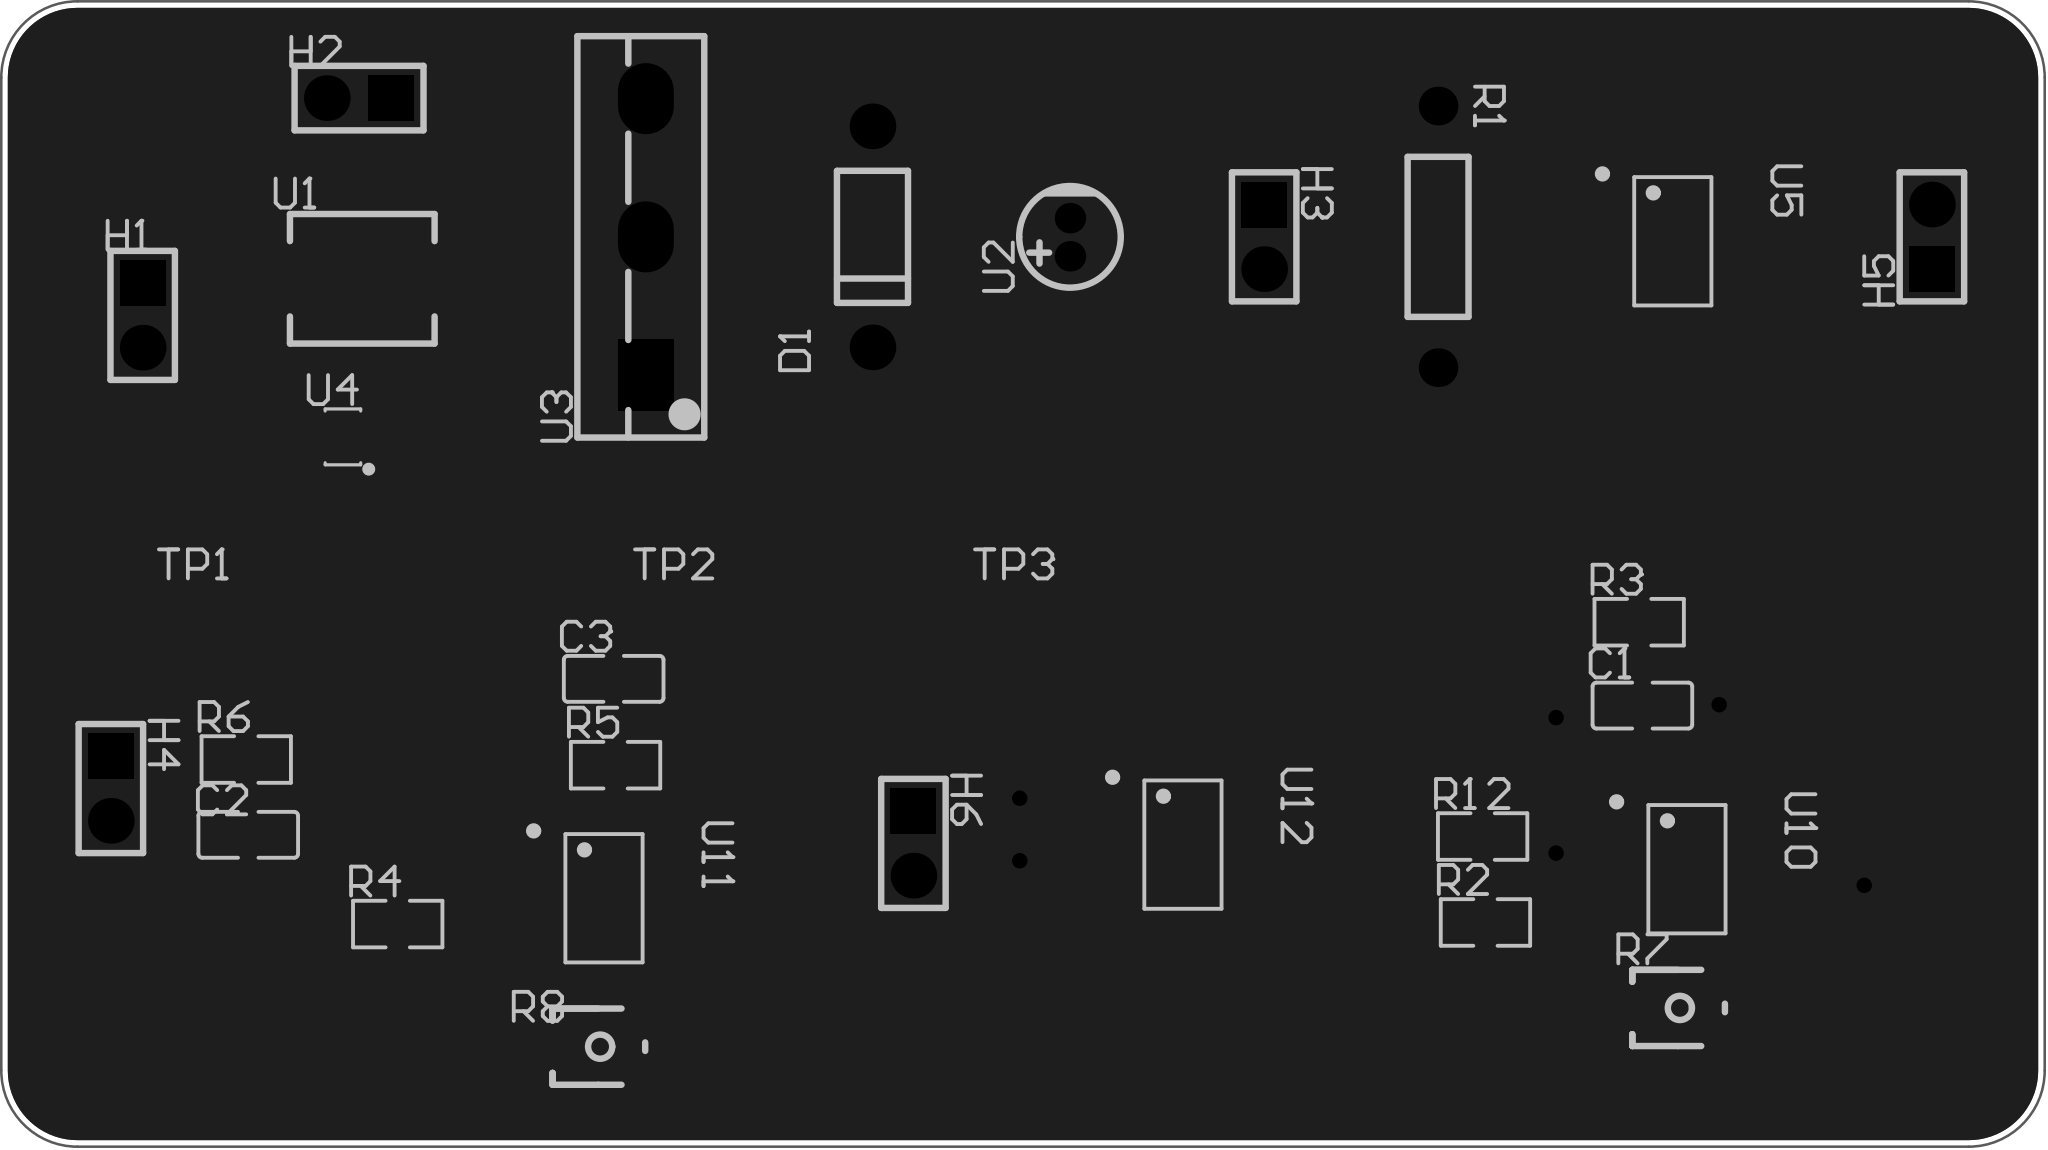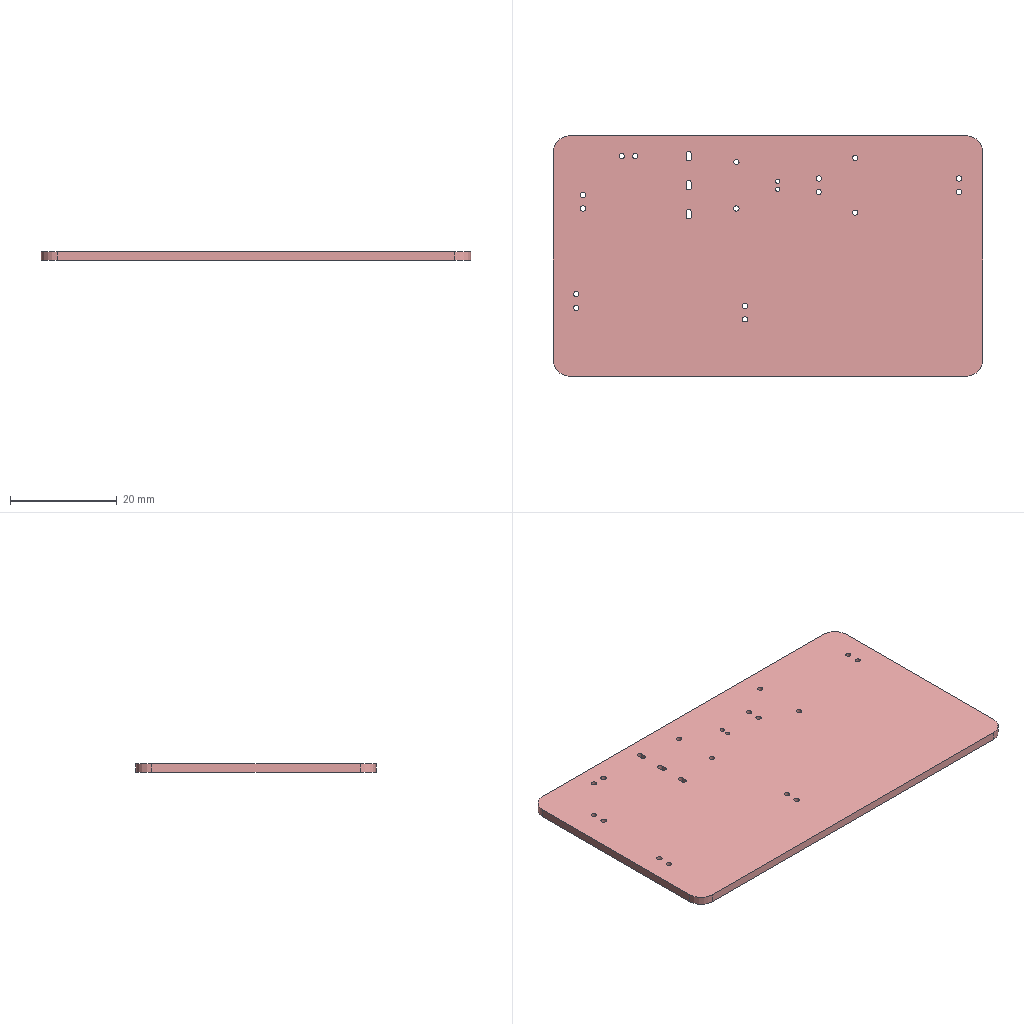Circuit board layout | Altium Designer | box 80.5 x 45.1 x 1.6 mm
Layer stack:
# Altium Designer layer stack of  (unit mm; dielectric type: 0 none, 1 core, 2 prepreg, 3 surface material)
index,name,kind,layer,copper_thickness_mm,dielectric_type,dielectric_thickness_mm,dielectric_material,dielectric_constant
0,Top Paste Mask Layer,other,,,,,,
1,Top Silkscreen Layer,other,,,,,,
2,Top Solder Mask Layer,dielectric,,,3,0.01,,3.3
3,Top Layer,copper,Top Layer,0.035,,,,
4,Dielectric1,dielectric,,,3,1.51,FR4,4.5
5,Bottom Layer,copper,Bottom Layer,0.035,,,,
6,Bottom Solder Mask Layer,dielectric,,,3,0.01,,3.3
7,Bottom Silkscreen Layer,other,,,,,,
8,Bottom Paste Mask Layer,other,,,,,,
# drill layer pairs: low layer,high layer
drill_pair,Top Layer,Bottom Layer
Part placement:
Designator,Comment,Layer,Footprint,Center-X(mm),Center-Y(mm),Rotation
C1,100nF,TopLayer,C0805,143.405,96.103,0
C2,100nF,TopLayer,C0805,88.471,91.017,180
C3,1nF,TopLayer,C0805,102.87,97.155,0
D1,,TopLayer,DO_1N4007,113.068,114.554,90
H1,,TopLayer,HDR-TH_2P-P2.54-V-M-1,84.312,111.462,270
H2,,TopLayer,HDR-TH_2P-P2.54-V-M-1,92.837,120.015,180
H3,,TopLayer,HDR-TH_2P-P2.54-V-M-1,128.502,114.554,270
H4,,TopLayer,HDR-TH_2P-P2.54-V-M-1,83.058,92.837,270
H5,,TopLayer,HDR-TH_2P-P2.54-V-M-1,154.813,114.554,90
H6,,TopLayer,HDR-TH_2P-P2.54-V-M-1,114.681,90.678,270
R1,10kΩ,TopLayer,Res_1/4W,135.354,114.554,270
R2,10kΩ,TopLayer,R0805,137.221,87.566,0
R3,1MΩ,TopLayer,R0805,143.278,99.385,0
R4,10kΩ,TopLayer,R0805,94.361,87.503,0
R5,10kΩ,TopLayer,R0805,102.945,93.757,0
R6,100Ω,TopLayer,R0805,88.392,93.98,0
R7,100kΩ,TopLayer,RES-ADJ-SMD_VG039NCH,144.907,84.201,0
R8,100kΩ,TopLayer,RES-ADJ-SMD_VG039NCH,102.362,82.677,0
R12,10kΩ,TopLayer,R0805,137.111,90.949,0
TP1,,TopLayer,Test-Point-0.5mm,85.201,100.731,0
TP2,,TopLayer,Test-Point-0.5mm,103.961,100.731,0
TP3,,TopLayer,Test-Point-0.5mm,117.358,100.731,0
U1,Power inductor (SMD),CKST0502-10uH/M,10uH,±20%,3A,package 5.7mm*5.1mm*2.0mm,CENKER,RoHS,TopLayer,IND-SMD_L5.7-W5.1,92.964,112.903,0
U2,10uF,TopLayer,CAP-TH_BD4.0-P1.50-D0.8-FD,120.849,114.539,90
U3,HY5204,TopLayer,TO-247-3_L15.8-W5.0-P5.44-L-1,104.14,114.554,90
U4,SN74LVC2G04DCKR,TopLayer,SOT-363_L2.0-W1.3-P0.65-LS2.1-BR,92.202,106.68,0
U5,NE5532DR,TopLayer,SOIC-8_L4.9-W3.9-P1.27-LS6.0-BL,144.604,114.379,270
U10,UA741CDT,TopLayer,SOIC-8_L4.9-W3.9-P1.27-LS6.0-BL,145.161,89.662,270
U11,UA741CDT,TopLayer,SOIC-8_L4.9-W3.9-P1.27-LS6.0-BL,102.489,88.519,270
U12,NE5532DR,TopLayer,SOIC-8_L4.9-W3.9-P1.27-LS6.0-BL,125.301,90.63,270
Pad and via stacks:
# Altium Designer via and pad stacks of  (unit mm). Each distinct definition once, with the count of objects using it.
# via: kind,start_layer,end_layer,hole_mm,diameter_mm,mode(0 simple;1 top-mid-bottom;2 full stack),diameter_per_layer,count,example_net
# pad: kind,layer,hole_mm,hole_type(0 round;1 square;2 slot),plating,top_size,top_shape(1 round;2 rect;3 octagon;9 rounded rect),mid_size,bottom_size,mode,footprint,size_per_layer,count,example
pad,Top Layer,0,0,plated,1.41x1.35,2,1.41x1.35,1.41x1.35,0,C0805,,6,C1.2
pad,Top Layer,0,0,plated,1.133x1.377,2,1.133x1.377,1.133x1.377,0,R0805,,12,R2.2
pad,Top Layer,0,0,plated,1.6x1.6,2,1.6x1.6,1.6x1.6,0,RES-ADJ-SMD_VG039NCH,,2,R7.2
pad,Top Layer,0,0,plated,1.2x1.5,2,1.2x1.5,1.2x1.5,0,RES-ADJ-SMD_VG039NCH,,4,R7.3
pad,Top Layer,0,0,plated,0.5x0.5,1,0.5x0.5,0.5x0.5,0,Test-Point-0.5mm,,3,TP1.1
pad,Top Layer,0,0,plated,2x2.5,2,2x2.5,2x2.5,0,IND-SMD_L5.7-W5.1,,2,U1.1
pad,Top Layer,0,0,plated,0.4x0.9,2,0.4x0.9,0.4x0.9,0,SOT-363_L2.0-W1.3-P0.65-LS2.1-BR,,6,U4.2
pad,Top Layer,0,0,plated,0.588x2.045,1,0.588x2.045,0.588x2.045,0,SOIC-8_L4.9-W3.9-P1.27-LS6.0-BL,,32,U5.1
pad,Multi-Layer,1,0,plated,1.8x1.8,1,1.8x1.8,1.8x1.8,0,DO_1N4007,,2,D1.1
pad,Multi-Layer,1,0,plated,1.8x1.8,1,1.8x1.8,1.8x1.8,0,HDR-TH_2P-P2.54-V-M-1,,6,H1.2
pad,Multi-Layer,1,0,plated,1.8x1.8,2,1.8x1.8,1.8x1.8,0,HDR-TH_2P-P2.54-V-M-1,,6,H1.1
pad,Multi-Layer,1,0,plated,1.524x1.524,1,1.524x1.524,1.524x1.524,0,Res_1/4W,,2,R1.1
pad,Multi-Layer,0.8,0,plated,1.2x1.2,1,1.2x1.2,1.2x1.2,0,CAP-TH_BD4.0-P1.50-D0.8-FD,,2,U2.2
pad,Multi-Layer,1,2,plated,2.8x2.2,1,2.8x2.2,2.8x2.2,0,TO-247-3_L15.8-W5.0-P5.44-L-1,,2,U3.3
pad,Multi-Layer,1,2,plated,2.8x2.2,2,2.8x2.2,2.8x2.2,0,TO-247-3_L15.8-W5.0-P5.44-L-1,,1,U3.1
via,Top Layer,Bottom Layer,0.3048,0.6096,0,,5,$1N3432
via,Top Layer,Bottom Layer,0.3048,0.61,0,,1,$1N3429
Copper pours:
name,layer,net,type(0 solid;1 hatched;2 none)
Top Layer-GND,Top Layer,GND,0
Bottom Layer-GND,Bottom Layer,GND,0